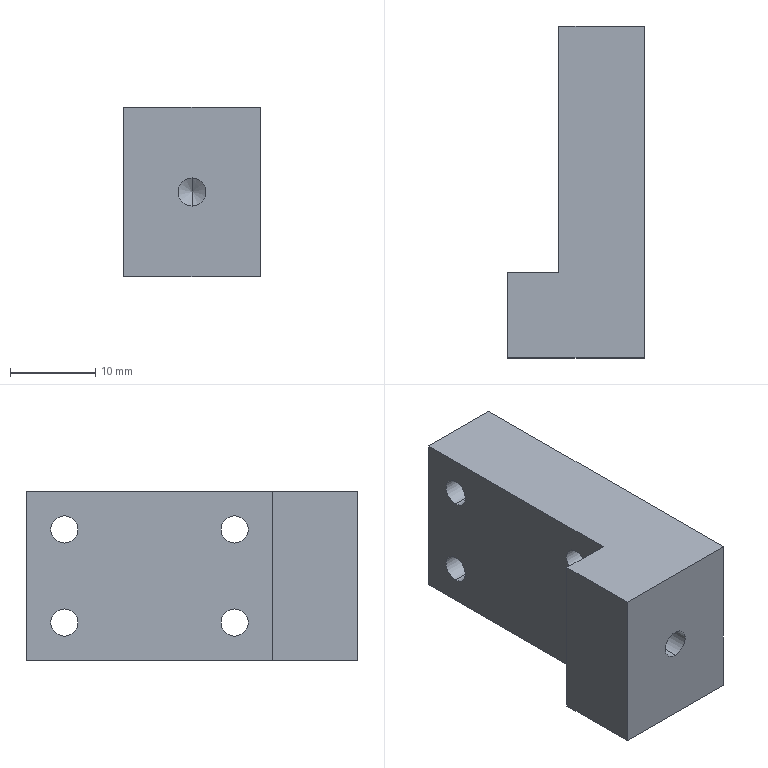Part | NX | features BREP 1 | 1 solid | 32 faces | box 16 x 39 x 19.94 mm | volume 8238 mm3 | cylinder 18 | plane 12 | cone 2 | commonest cylinder face diameters 3.2 x8 6.5 x8 3.3 x2
STEP:
#1=CARTESIAN_POINT('',(-8.,9.,11.62));
#2=VERTEX_POINT('',#1);
#3=CARTESIAN_POINT('',(-8.,9.,8.32));
#4=VERTEX_POINT('',#3);
#5=CARTESIAN_POINT('',(-8.,9.,9.97));
#6=DIRECTION('',(0.,-1.,0.));
#7=DIRECTION('',(0.,0.,-1.));
#8=AXIS2_PLACEMENT_3D('',#5,#6,#7);
#9=CIRCLE('',#8,1.65);
#10=EDGE_CURVE('',#2,#4,#9,.T.);
#11=ORIENTED_EDGE('',*,*,#10,.F.);
#12=CARTESIAN_POINT('',(-8.,1.,11.62));
#13=VERTEX_POINT('',#12);
#14=CARTESIAN_POINT('',(-8.,1.,11.62));
#15=DIRECTION('',(0.,-1.,0.));
#16=VECTOR('',#15,1000.);
#17=LINE('',#14,#16);
#18=EDGE_CURVE('',#2,#13,#17,.T.);
#19=ORIENTED_EDGE('',*,*,#18,.T.);
#20=CARTESIAN_POINT('',(-8.,1.,8.32));
#21=VERTEX_POINT('',#20);
#22=CARTESIAN_POINT('',(-8.,1.,9.97));
#23=DIRECTION('',(0.,-1.,0.));
#24=DIRECTION('',(0.,0.,-1.));
#25=AXIS2_PLACEMENT_3D('',#22,#23,#24);
#26=CIRCLE('',#25,1.65);
#27=EDGE_CURVE('',#13,#21,#26,.T.);
#28=ORIENTED_EDGE('',*,*,#27,.T.);
#29=CARTESIAN_POINT('',(-8.,1.,8.32));
#30=DIRECTION('',(0.,-1.,0.));
#31=VECTOR('',#30,1000.);
#32=LINE('',#29,#31);
#33=EDGE_CURVE('',#4,#21,#32,.T.);
#34=ORIENTED_EDGE('',*,*,#33,.F.);
#35=EDGE_LOOP('',(#11,#19,#28,#34));
#36=FACE_BOUND('',#35,.T.);
#37=CARTESIAN_POINT('',(-8.,1.,9.97));
#38=DIRECTION('',(0.,-1.,0.));
#39=DIRECTION('',(0.,0.,-1.));
#40=AXIS2_PLACEMENT_3D('',#37,#38,#39);
#41=CYLINDRICAL_SURFACE('',#40,1.65);
#42=ADVANCED_FACE('',(#36),#41,.F.);
#43=CARTESIAN_POINT('',(-8.,9.991,9.97));
#44=VERTEX_POINT('',#43);
#45=CARTESIAN_POINT('',(-8.,9.,8.32));
#46=DIRECTION('',(0.,-0.515,-0.8572));
#47=VECTOR('',#46,1000.);
#48=LINE('',#45,#47);
#49=EDGE_CURVE('',#44,#4,#48,.T.);
#50=ORIENTED_EDGE('',*,*,#49,.F.);
#51=CARTESIAN_POINT('',(-8.,9.,11.62));
#52=DIRECTION('',(0.,-0.515,0.8572));
#53=VECTOR('',#52,1000.);
#54=LINE('',#51,#53);
#55=EDGE_CURVE('',#44,#2,#54,.T.);
#56=ORIENTED_EDGE('',*,*,#55,.T.);
#57=ORIENTED_EDGE('',*,*,#10,.T.);
#58=EDGE_LOOP('',(#50,#56,#57));
#59=FACE_BOUND('',#58,.T.);
#60=CARTESIAN_POINT('',(-8.,9.,9.97));
#61=DIRECTION('',(0.,-1.,0.));
#62=DIRECTION('',(0.,0.,-1.));
#63=AXIS2_PLACEMENT_3D('',#60,#61,#62);
#64=CONICAL_SURFACE('',#63,1.65,1.03);
#65=ADVANCED_FACE('',(#59),#64,.F.);
#66=CARTESIAN_POINT('',(-3.4,35.5,18.69));
#67=VERTEX_POINT('',#66);
#68=CARTESIAN_POINT('',(-3.4,35.5,12.19));
#69=VERTEX_POINT('',#68);
#70=CARTESIAN_POINT('',(-3.4,35.5,15.44));
#71=DIRECTION('',(1.,0.,0.));
#72=DIRECTION('',(0.,0.,-1.));
#73=AXIS2_PLACEMENT_3D('',#70,#71,#72);
#74=CIRCLE('',#73,3.25);
#75=EDGE_CURVE('',#67,#69,#74,.T.);
#76=ORIENTED_EDGE('',*,*,#75,.F.);
#77=CARTESIAN_POINT('',(0.,35.5,18.69));
#78=VERTEX_POINT('',#77);
#79=CARTESIAN_POINT('',(0.,35.5,18.69));
#80=DIRECTION('',(1.,0.,0.));
#81=VECTOR('',#80,1000.);
#82=LINE('',#79,#81);
#83=EDGE_CURVE('',#67,#78,#82,.T.);
#84=ORIENTED_EDGE('',*,*,#83,.T.);
#85=CARTESIAN_POINT('',(0.,35.5,12.19));
#86=VERTEX_POINT('',#85);
#87=CARTESIAN_POINT('',(0.,35.5,15.44));
#88=DIRECTION('',(1.,0.,0.));
#89=DIRECTION('',(0.,0.,-1.));
#90=AXIS2_PLACEMENT_3D('',#87,#88,#89);
#91=CIRCLE('',#90,3.25);
#92=EDGE_CURVE('',#78,#86,#91,.T.);
#93=ORIENTED_EDGE('',*,*,#92,.T.);
#94=CARTESIAN_POINT('',(0.,35.5,12.19));
#95=DIRECTION('',(1.,0.,0.));
#96=VECTOR('',#95,1000.);
#97=LINE('',#94,#96);
#98=EDGE_CURVE('',#69,#86,#97,.T.);
#99=ORIENTED_EDGE('',*,*,#98,.F.);
#100=EDGE_LOOP('',(#76,#84,#93,#99));
#101=FACE_BOUND('',#100,.T.);
#102=CARTESIAN_POINT('',(0.,35.5,15.44));
#103=DIRECTION('',(1.,0.,0.));
#104=DIRECTION('',(0.,0.,-1.));
#105=AXIS2_PLACEMENT_3D('',#102,#103,#104);
#106=CYLINDRICAL_SURFACE('',#105,3.25);
#107=ADVANCED_FACE('',(#101),#106,.F.);
#108=CARTESIAN_POINT('',(-10.,35.5,17.04));
#109=VERTEX_POINT('',#108);
#110=CARTESIAN_POINT('',(-10.,35.5,13.84));
#111=VERTEX_POINT('',#110);
#112=CARTESIAN_POINT('',(-10.,35.5,15.44));
#113=DIRECTION('',(1.,0.,0.));
#114=DIRECTION('',(0.,0.,-1.));
#115=AXIS2_PLACEMENT_3D('',#112,#113,#114);
#116=CIRCLE('',#115,1.6);
#117=EDGE_CURVE('',#109,#111,#116,.T.);
#118=ORIENTED_EDGE('',*,*,#117,.F.);
#119=CARTESIAN_POINT('',(-3.4,35.5,17.04));
#120=VERTEX_POINT('',#119);
#121=CARTESIAN_POINT('',(0.,35.5,17.04));
#122=DIRECTION('',(1.,0.,0.));
#123=VECTOR('',#122,1000.);
#124=LINE('',#121,#123);
#125=EDGE_CURVE('',#109,#120,#124,.T.);
#126=ORIENTED_EDGE('',*,*,#125,.T.);
#127=CARTESIAN_POINT('',(-3.4,35.5,13.84));
#128=VERTEX_POINT('',#127);
#129=CARTESIAN_POINT('',(-3.4,35.5,15.44));
#130=DIRECTION('',(1.,0.,0.));
#131=DIRECTION('',(0.,0.,-1.));
#132=AXIS2_PLACEMENT_3D('',#129,#130,#131);
#133=CIRCLE('',#132,1.6);
#134=EDGE_CURVE('',#120,#128,#133,.T.);
#135=ORIENTED_EDGE('',*,*,#134,.T.);
#136=CARTESIAN_POINT('',(0.,35.5,13.84));
#137=DIRECTION('',(1.,0.,0.));
#138=VECTOR('',#137,1000.);
#139=LINE('',#136,#138);
#140=EDGE_CURVE('',#111,#128,#139,.T.);
#141=ORIENTED_EDGE('',*,*,#140,.F.);
#142=EDGE_LOOP('',(#118,#126,#135,#141));
#143=FACE_BOUND('',#142,.T.);
#144=CARTESIAN_POINT('',(0.,35.5,15.44));
#145=DIRECTION('',(1.,0.,0.));
#146=DIRECTION('',(0.,0.,-1.));
#147=AXIS2_PLACEMENT_3D('',#144,#145,#146);
#148=CYLINDRICAL_SURFACE('',#147,1.6);
#149=ADVANCED_FACE('',(#143),#148,.F.);
#150=CARTESIAN_POINT('',(-3.4,15.5,18.69));
#151=VERTEX_POINT('',#150);
#152=CARTESIAN_POINT('',(-3.4,15.5,12.19));
#153=VERTEX_POINT('',#152);
#154=CARTESIAN_POINT('',(-3.4,15.5,15.44));
#155=DIRECTION('',(1.,0.,0.));
#156=DIRECTION('',(0.,0.,-1.));
#157=AXIS2_PLACEMENT_3D('',#154,#155,#156);
#158=CIRCLE('',#157,3.25);
#159=EDGE_CURVE('',#151,#153,#158,.T.);
#160=ORIENTED_EDGE('',*,*,#159,.F.);
#161=CARTESIAN_POINT('',(0.,15.5,18.69));
#162=VERTEX_POINT('',#161);
#163=CARTESIAN_POINT('',(0.,15.5,18.69));
#164=DIRECTION('',(1.,0.,0.));
#165=VECTOR('',#164,1000.);
#166=LINE('',#163,#165);
#167=EDGE_CURVE('',#151,#162,#166,.T.);
#168=ORIENTED_EDGE('',*,*,#167,.T.);
#169=CARTESIAN_POINT('',(0.,15.5,12.19));
#170=VERTEX_POINT('',#169);
#171=CARTESIAN_POINT('',(0.,15.5,15.44));
#172=DIRECTION('',(1.,0.,0.));
#173=DIRECTION('',(0.,0.,-1.));
#174=AXIS2_PLACEMENT_3D('',#171,#172,#173);
#175=CIRCLE('',#174,3.25);
#176=EDGE_CURVE('',#162,#170,#175,.T.);
#177=ORIENTED_EDGE('',*,*,#176,.T.);
#178=CARTESIAN_POINT('',(0.,15.5,12.19));
#179=DIRECTION('',(1.,0.,0.));
#180=VECTOR('',#179,1000.);
#181=LINE('',#178,#180);
#182=EDGE_CURVE('',#153,#170,#181,.T.);
#183=ORIENTED_EDGE('',*,*,#182,.F.);
#184=EDGE_LOOP('',(#160,#168,#177,#183));
#185=FACE_BOUND('',#184,.T.);
#186=CARTESIAN_POINT('',(0.,15.5,15.44));
#187=DIRECTION('',(1.,0.,0.));
#188=DIRECTION('',(0.,0.,-1.));
#189=AXIS2_PLACEMENT_3D('',#186,#187,#188);
#190=CYLINDRICAL_SURFACE('',#189,3.25);
#191=ADVANCED_FACE('',(#185),#190,.F.);
#192=CARTESIAN_POINT('',(-10.,15.5,17.04));
#193=VERTEX_POINT('',#192);
#194=CARTESIAN_POINT('',(-10.,15.5,13.84));
#195=VERTEX_POINT('',#194);
#196=CARTESIAN_POINT('',(-10.,15.5,15.44));
#197=DIRECTION('',(1.,0.,0.));
#198=DIRECTION('',(0.,0.,-1.));
#199=AXIS2_PLACEMENT_3D('',#196,#197,#198);
#200=CIRCLE('',#199,1.6);
#201=EDGE_CURVE('',#193,#195,#200,.T.);
#202=ORIENTED_EDGE('',*,*,#201,.F.);
#203=CARTESIAN_POINT('',(-3.4,15.5,17.04));
#204=VERTEX_POINT('',#203);
#205=CARTESIAN_POINT('',(0.,15.5,17.04));
#206=DIRECTION('',(1.,0.,0.));
#207=VECTOR('',#206,1000.);
#208=LINE('',#205,#207);
#209=EDGE_CURVE('',#193,#204,#208,.T.);
#210=ORIENTED_EDGE('',*,*,#209,.T.);
#211=CARTESIAN_POINT('',(-3.4,15.5,13.84));
#212=VERTEX_POINT('',#211);
#213=CARTESIAN_POINT('',(-3.4,15.5,15.44));
#214=DIRECTION('',(1.,0.,0.));
#215=DIRECTION('',(0.,0.,-1.));
#216=AXIS2_PLACEMENT_3D('',#213,#214,#215);
#217=CIRCLE('',#216,1.6);
#218=EDGE_CURVE('',#204,#212,#217,.T.);
#219=ORIENTED_EDGE('',*,*,#218,.T.);
#220=CARTESIAN_POINT('',(0.,15.5,13.84));
#221=DIRECTION('',(1.,0.,0.));
#222=VECTOR('',#221,1000.);
#223=LINE('',#220,#222);
#224=EDGE_CURVE('',#195,#212,#223,.T.);
#225=ORIENTED_EDGE('',*,*,#224,.F.);
#226=EDGE_LOOP('',(#202,#210,#219,#225));
#227=FACE_BOUND('',#226,.T.);
#228=CARTESIAN_POINT('',(0.,15.5,15.44));
#229=DIRECTION('',(1.,0.,0.));
#230=DIRECTION('',(0.,0.,-1.));
#231=AXIS2_PLACEMENT_3D('',#228,#229,#230);
#232=CYLINDRICAL_SURFACE('',#231,1.6);
#233=ADVANCED_FACE('',(#227),#232,.F.);
#234=CARTESIAN_POINT('',(-3.4,35.5,7.75));
#235=VERTEX_POINT('',#234);
#236=CARTESIAN_POINT('',(-3.4,35.5,1.25));
#237=VERTEX_POINT('',#236);
#238=CARTESIAN_POINT('',(-3.4,35.5,4.5));
#239=DIRECTION('',(1.,0.,0.));
#240=DIRECTION('',(0.,0.,-1.));
#241=AXIS2_PLACEMENT_3D('',#238,#239,#240);
#242=CIRCLE('',#241,3.25);
#243=EDGE_CURVE('',#235,#237,#242,.T.);
#244=ORIENTED_EDGE('',*,*,#243,.F.);
#245=CARTESIAN_POINT('',(0.,35.5,7.75));
#246=VERTEX_POINT('',#245);
#247=CARTESIAN_POINT('',(0.,35.5,7.75));
#248=DIRECTION('',(1.,0.,0.));
#249=VECTOR('',#248,1000.);
#250=LINE('',#247,#249);
#251=EDGE_CURVE('',#235,#246,#250,.T.);
#252=ORIENTED_EDGE('',*,*,#251,.T.);
#253=CARTESIAN_POINT('',(0.,35.5,1.25));
#254=VERTEX_POINT('',#253);
#255=CARTESIAN_POINT('',(0.,35.5,4.5));
#256=DIRECTION('',(1.,0.,0.));
#257=DIRECTION('',(0.,0.,-1.));
#258=AXIS2_PLACEMENT_3D('',#255,#256,#257);
#259=CIRCLE('',#258,3.25);
#260=EDGE_CURVE('',#246,#254,#259,.T.);
#261=ORIENTED_EDGE('',*,*,#260,.T.);
#262=CARTESIAN_POINT('',(0.,35.5,1.25));
#263=DIRECTION('',(1.,0.,0.));
#264=VECTOR('',#263,1000.);
#265=LINE('',#262,#264);
#266=EDGE_CURVE('',#237,#254,#265,.T.);
#267=ORIENTED_EDGE('',*,*,#266,.F.);
#268=EDGE_LOOP('',(#244,#252,#261,#267));
#269=FACE_BOUND('',#268,.T.);
#270=CARTESIAN_POINT('',(0.,35.5,4.5));
#271=DIRECTION('',(1.,0.,0.));
#272=DIRECTION('',(0.,0.,-1.));
#273=AXIS2_PLACEMENT_3D('',#270,#271,#272);
#274=CYLINDRICAL_SURFACE('',#273,3.25);
#275=ADVANCED_FACE('',(#269),#274,.F.);
#276=CARTESIAN_POINT('',(-10.,35.5,6.1));
#277=VERTEX_POINT('',#276);
#278=CARTESIAN_POINT('',(-10.,35.5,2.9));
#279=VERTEX_POINT('',#278);
#280=CARTESIAN_POINT('',(-10.,35.5,4.5));
#281=DIRECTION('',(1.,0.,0.));
#282=DIRECTION('',(0.,0.,-1.));
#283=AXIS2_PLACEMENT_3D('',#280,#281,#282);
#284=CIRCLE('',#283,1.6);
#285=EDGE_CURVE('',#277,#279,#284,.T.);
#286=ORIENTED_EDGE('',*,*,#285,.F.);
#287=CARTESIAN_POINT('',(-3.4,35.5,6.1));
#288=VERTEX_POINT('',#287);
#289=CARTESIAN_POINT('',(0.,35.5,6.1));
#290=DIRECTION('',(1.,0.,0.));
#291=VECTOR('',#290,1000.);
#292=LINE('',#289,#291);
#293=EDGE_CURVE('',#277,#288,#292,.T.);
#294=ORIENTED_EDGE('',*,*,#293,.T.);
#295=CARTESIAN_POINT('',(-3.4,35.5,2.9));
#296=VERTEX_POINT('',#295);
#297=CARTESIAN_POINT('',(-3.4,35.5,4.5));
#298=DIRECTION('',(1.,0.,0.));
#299=DIRECTION('',(0.,0.,-1.));
#300=AXIS2_PLACEMENT_3D('',#297,#298,#299);
#301=CIRCLE('',#300,1.6);
#302=EDGE_CURVE('',#288,#296,#301,.T.);
#303=ORIENTED_EDGE('',*,*,#302,.T.);
#304=CARTESIAN_POINT('',(0.,35.5,2.9));
#305=DIRECTION('',(1.,0.,0.));
#306=VECTOR('',#305,1000.);
#307=LINE('',#304,#306);
#308=EDGE_CURVE('',#279,#296,#307,.T.);
#309=ORIENTED_EDGE('',*,*,#308,.F.);
#310=EDGE_LOOP('',(#286,#294,#303,#309));
#311=FACE_BOUND('',#310,.T.);
#312=CARTESIAN_POINT('',(0.,35.5,4.5));
#313=DIRECTION('',(1.,0.,0.));
#314=DIRECTION('',(0.,0.,-1.));
#315=AXIS2_PLACEMENT_3D('',#312,#313,#314);
#316=CYLINDRICAL_SURFACE('',#315,1.6);
#317=ADVANCED_FACE('',(#311),#316,.F.);
#318=CARTESIAN_POINT('',(-3.4,15.5,7.75));
#319=VERTEX_POINT('',#318);
#320=CARTESIAN_POINT('',(-3.4,15.5,1.25));
#321=VERTEX_POINT('',#320);
#322=CARTESIAN_POINT('',(-3.4,15.5,4.5));
#323=DIRECTION('',(1.,0.,0.));
#324=DIRECTION('',(0.,0.,-1.));
#325=AXIS2_PLACEMENT_3D('',#322,#323,#324);
#326=CIRCLE('',#325,3.25);
#327=EDGE_CURVE('',#319,#321,#326,.T.);
#328=ORIENTED_EDGE('',*,*,#327,.F.);
#329=CARTESIAN_POINT('',(0.,15.5,7.75));
#330=VERTEX_POINT('',#329);
#331=CARTESIAN_POINT('',(0.,15.5,7.75));
#332=DIRECTION('',(1.,0.,0.));
#333=VECTOR('',#332,1000.);
#334=LINE('',#331,#333);
#335=EDGE_CURVE('',#319,#330,#334,.T.);
#336=ORIENTED_EDGE('',*,*,#335,.T.);
#337=CARTESIAN_POINT('',(0.,15.5,1.25));
#338=VERTEX_POINT('',#337);
#339=CARTESIAN_POINT('',(0.,15.5,4.5));
#340=DIRECTION('',(1.,0.,0.));
#341=DIRECTION('',(0.,0.,-1.));
#342=AXIS2_PLACEMENT_3D('',#339,#340,#341);
#343=CIRCLE('',#342,3.25);
#344=EDGE_CURVE('',#330,#338,#343,.T.);
#345=ORIENTED_EDGE('',*,*,#344,.T.);
#346=CARTESIAN_POINT('',(0.,15.5,1.25));
#347=DIRECTION('',(1.,0.,0.));
#348=VECTOR('',#347,1000.);
#349=LINE('',#346,#348);
#350=EDGE_CURVE('',#321,#338,#349,.T.);
#351=ORIENTED_EDGE('',*,*,#350,.F.);
#352=EDGE_LOOP('',(#328,#336,#345,#351));
#353=FACE_BOUND('',#352,.T.);
#354=CARTESIAN_POINT('',(0.,15.5,4.5));
#355=DIRECTION('',(1.,0.,0.));
#356=DIRECTION('',(0.,0.,-1.));
#357=AXIS2_PLACEMENT_3D('',#354,#355,#356);
#358=CYLINDRICAL_SURFACE('',#357,3.25);
#359=ADVANCED_FACE('',(#353),#358,.F.);
#360=CARTESIAN_POINT('',(-10.,15.5,6.1));
#361=VERTEX_POINT('',#360);
#362=CARTESIAN_POINT('',(-10.,15.5,2.9));
#363=VERTEX_POINT('',#362);
#364=CARTESIAN_POINT('',(-10.,15.5,4.5));
#365=DIRECTION('',(1.,0.,0.));
#366=DIRECTION('',(0.,0.,-1.));
#367=AXIS2_PLACEMENT_3D('',#364,#365,#366);
#368=CIRCLE('',#367,1.6);
#369=EDGE_CURVE('',#361,#363,#368,.T.);
#370=ORIENTED_EDGE('',*,*,#369,.F.);
#371=CARTESIAN_POINT('',(-3.4,15.5,6.1));
#372=VERTEX_POINT('',#371);
#373=CARTESIAN_POINT('',(0.,15.5,6.1));
#374=DIRECTION('',(1.,0.,0.));
#375=VECTOR('',#374,1000.);
#376=LINE('',#373,#375);
#377=EDGE_CURVE('',#361,#372,#376,.T.);
#378=ORIENTED_EDGE('',*,*,#377,.T.);
#379=CARTESIAN_POINT('',(-3.4,15.5,2.9));
#380=VERTEX_POINT('',#379);
#381=CARTESIAN_POINT('',(-3.4,15.5,4.5));
#382=DIRECTION('',(1.,0.,0.));
#383=DIRECTION('',(0.,0.,-1.));
#384=AXIS2_PLACEMENT_3D('',#381,#382,#383);
#385=CIRCLE('',#384,1.6);
#386=EDGE_CURVE('',#372,#380,#385,.T.);
#387=ORIENTED_EDGE('',*,*,#386,.T.);
#388=CARTESIAN_POINT('',(0.,15.5,2.9));
#389=DIRECTION('',(1.,0.,0.));
#390=VECTOR('',#389,1000.);
#391=LINE('',#388,#390);
#392=EDGE_CURVE('',#363,#380,#391,.T.);
#393=ORIENTED_EDGE('',*,*,#392,.F.);
#394=EDGE_LOOP('',(#370,#378,#387,#393));
#395=FACE_BOUND('',#394,.T.);
#396=CARTESIAN_POINT('',(0.,15.5,4.5));
#397=DIRECTION('',(1.,0.,0.));
#398=DIRECTION('',(0.,0.,-1.));
#399=AXIS2_PLACEMENT_3D('',#396,#397,#398);
#400=CYLINDRICAL_SURFACE('',#399,1.6);
#401=ADVANCED_FACE('',(#395),#400,.F.);
#402=CARTESIAN_POINT('',(0.,1.,0.));
#403=VERTEX_POINT('',#402);
#404=CARTESIAN_POINT('',(0.,1.,19.94));
#405=VERTEX_POINT('',#404);
#406=CARTESIAN_POINT('',(0.,1.,19.94));
#407=DIRECTION('',(0.,0.,1.));
#408=VECTOR('',#407,1000.);
#409=LINE('',#406,#408);
#410=EDGE_CURVE('',#403,#405,#409,.T.);
#411=ORIENTED_EDGE('',*,*,#410,.F.);
#412=CARTESIAN_POINT('',(0.,40.,0.));
#413=VERTEX_POINT('',#412);
#414=CARTESIAN_POINT('',(0.,0.,0.));
#415=DIRECTION('',(0.,-1.,0.));
#416=VECTOR('',#415,1000.);
#417=LINE('',#414,#416);
#418=EDGE_CURVE('',#413,#403,#417,.T.);
#419=ORIENTED_EDGE('',*,*,#418,.F.);
#420=CARTESIAN_POINT('',(0.,40.,19.94));
#421=VERTEX_POINT('',#420);
#422=CARTESIAN_POINT('',(0.,40.,19.94));
#423=DIRECTION('',(0.,0.,-1.));
#424=VECTOR('',#423,1000.);
#425=LINE('',#422,#424);
#426=EDGE_CURVE('',#421,#413,#425,.T.);
#427=ORIENTED_EDGE('',*,*,#426,.F.);
#428=CARTESIAN_POINT('',(0.,0.,19.94));
#429=DIRECTION('',(0.,-1.,0.));
#430=VECTOR('',#429,1000.);
#431=LINE('',#428,#430);
#432=EDGE_CURVE('',#421,#405,#431,.T.);
#433=ORIENTED_EDGE('',*,*,#432,.T.);
#434=EDGE_LOOP('',(#411,#419,#427,#433));
#435=FACE_BOUND('',#434,.T.);
#436=CARTESIAN_POINT('',(0.,35.5,15.44));
#437=DIRECTION('',(1.,0.,0.));
#438=DIRECTION('',(0.,0.,-1.));
#439=AXIS2_PLACEMENT_3D('',#436,#437,#438);
#440=CIRCLE('',#439,3.25);
#441=EDGE_CURVE('',#86,#78,#440,.T.);
#442=ORIENTED_EDGE('',*,*,#441,.F.);
#443=ORIENTED_EDGE('',*,*,#92,.F.);
#444=EDGE_LOOP('',(#442,#443));
#445=FACE_BOUND('',#444,.T.);
#446=CARTESIAN_POINT('',(0.,15.5,15.44));
#447=DIRECTION('',(1.,0.,0.));
#448=DIRECTION('',(0.,0.,-1.));
#449=AXIS2_PLACEMENT_3D('',#446,#447,#448);
#450=CIRCLE('',#449,3.25);
#451=EDGE_CURVE('',#170,#162,#450,.T.);
#452=ORIENTED_EDGE('',*,*,#451,.F.);
#453=ORIENTED_EDGE('',*,*,#176,.F.);
#454=EDGE_LOOP('',(#452,#453));
#455=FACE_BOUND('',#454,.T.);
#456=CARTESIAN_POINT('',(0.,35.5,4.5));
#457=DIRECTION('',(1.,0.,0.));
#458=DIRECTION('',(0.,0.,-1.));
#459=AXIS2_PLACEMENT_3D('',#456,#457,#458);
#460=CIRCLE('',#459,3.25);
#461=EDGE_CURVE('',#254,#246,#460,.T.);
#462=ORIENTED_EDGE('',*,*,#461,.F.);
#463=ORIENTED_EDGE('',*,*,#260,.F.);
#464=EDGE_LOOP('',(#462,#463));
#465=FACE_BOUND('',#464,.T.);
#466=CARTESIAN_POINT('',(0.,15.5,4.5));
#467=DIRECTION('',(1.,0.,0.));
#468=DIRECTION('',(0.,0.,-1.));
#469=AXIS2_PLACEMENT_3D('',#466,#467,#468);
#470=CIRCLE('',#469,3.25);
#471=EDGE_CURVE('',#338,#330,#470,.T.);
#472=ORIENTED_EDGE('',*,*,#471,.F.);
#473=ORIENTED_EDGE('',*,*,#344,.F.);
#474=EDGE_LOOP('',(#472,#473));
#475=FACE_BOUND('',#474,.T.);
#476=CARTESIAN_POINT('',(0.,0.,19.94));
#477=DIRECTION('',(1.,0.,0.));
#478=DIRECTION('',(0.,1.,0.));
#479=AXIS2_PLACEMENT_3D('',#476,#477,#478);
#480=PLANE('',#479);
#481=ADVANCED_FACE('',(#435,#445,#455,#465,#475),#480,.T.);
#482=CARTESIAN_POINT('',(-10.,40.,19.94));
#483=VERTEX_POINT('',#482);
#484=CARTESIAN_POINT('',(-10.,40.,0.));
#485=VERTEX_POINT('',#484);
#486=CARTESIAN_POINT('',(-10.,40.,19.94));
#487=DIRECTION('',(0.,0.,-1.));
#488=VECTOR('',#487,1000.);
#489=LINE('',#486,#488);
#490=EDGE_CURVE('',#483,#485,#489,.T.);
#491=ORIENTED_EDGE('',*,*,#490,.F.);
#492=CARTESIAN_POINT('',(-10.,40.,19.94));
#493=DIRECTION('',(1.,0.,0.));
#494=VECTOR('',#493,1000.);
#495=LINE('',#492,#494);
#496=EDGE_CURVE('',#483,#421,#495,.T.);
#497=ORIENTED_EDGE('',*,*,#496,.T.);
#498=ORIENTED_EDGE('',*,*,#426,.T.);
#499=CARTESIAN_POINT('',(-10.,40.,0.));
#500=DIRECTION('',(1.,0.,0.));
#501=VECTOR('',#500,1000.);
#502=LINE('',#499,#501);
#503=EDGE_CURVE('',#485,#413,#502,.T.);
#504=ORIENTED_EDGE('',*,*,#503,.F.);
#505=EDGE_LOOP('',(#491,#497,#498,#504));
#506=FACE_BOUND('',#505,.T.);
#507=CARTESIAN_POINT('',(-10.,40.,19.94));
#508=DIRECTION('',(0.,1.,0.));
#509=DIRECTION('',(1.,0.,0.));
#510=AXIS2_PLACEMENT_3D('',#507,#508,#509);
#511=PLANE('',#510);
#512=ADVANCED_FACE('',(#506),#511,.T.);
#513=CARTESIAN_POINT('',(-16.,11.,0.));
#514=VERTEX_POINT('',#513);
#515=CARTESIAN_POINT('',(-16.,1.,0.));
#516=VERTEX_POINT('',#515);
#517=CARTESIAN_POINT('',(-16.,0.,0.));
#518=DIRECTION('',(0.,-1.,0.));
#519=VECTOR('',#518,1000.);
#520=LINE('',#517,#519);
#521=EDGE_CURVE('',#514,#516,#520,.T.);
#522=ORIENTED_EDGE('',*,*,#521,.T.);
#523=CARTESIAN_POINT('',(-16.,1.,19.94));
#524=VERTEX_POINT('',#523);
#525=CARTESIAN_POINT('',(-16.,1.,19.94));
#526=DIRECTION('',(0.,0.,1.));
#527=VECTOR('',#526,1000.);
#528=LINE('',#525,#527);
#529=EDGE_CURVE('',#516,#524,#528,.T.);
#530=ORIENTED_EDGE('',*,*,#529,.T.);
#531=CARTESIAN_POINT('',(-16.,11.,19.94));
#532=VERTEX_POINT('',#531);
#533=CARTESIAN_POINT('',(-16.,0.,19.94));
#534=DIRECTION('',(0.,-1.,0.));
#535=VECTOR('',#534,1000.);
#536=LINE('',#533,#535);
#537=EDGE_CURVE('',#532,#524,#536,.T.);
#538=ORIENTED_EDGE('',*,*,#537,.F.);
#539=CARTESIAN_POINT('',(-16.,11.,19.94));
#540=DIRECTION('',(0.,0.,-1.));
#541=VECTOR('',#540,1000.);
#542=LINE('',#539,#541);
#543=EDGE_CURVE('',#532,#514,#542,.T.);
#544=ORIENTED_EDGE('',*,*,#543,.T.);
#545=EDGE_LOOP('',(#522,#530,#538,#544));
#546=FACE_BOUND('',#545,.T.);
#547=CARTESIAN_POINT('',(-16.,0.,19.94));
#548=DIRECTION('',(1.,0.,0.));
#549=DIRECTION('',(0.,1.,0.));
#550=AXIS2_PLACEMENT_3D('',#547,#548,#549);
#551=PLANE('',#550);
#552=ADVANCED_FACE('',(#546),#551,.F.);
#553=ORIENTED_EDGE('',*,*,#537,.T.);
#554=CARTESIAN_POINT('',(-49.363,1.,19.94));
#555=DIRECTION('',(-1.,0.,0.));
#556=VECTOR('',#555,1000.);
#557=LINE('',#554,#556);
#558=EDGE_CURVE('',#405,#524,#557,.T.);
#559=ORIENTED_EDGE('',*,*,#558,.F.);
#560=ORIENTED_EDGE('',*,*,#432,.F.);
#561=ORIENTED_EDGE('',*,*,#496,.F.);
#562=CARTESIAN_POINT('',(-10.,11.,19.94));
#563=VERTEX_POINT('',#562);
#564=CARTESIAN_POINT('',(-10.,11.,19.94));
#565=DIRECTION('',(0.,1.,0.));
#566=VECTOR('',#565,1000.);
#567=LINE('',#564,#566);
#568=EDGE_CURVE('',#563,#483,#567,.T.);
#569=ORIENTED_EDGE('',*,*,#568,.F.);
#570=CARTESIAN_POINT('',(-6.,11.,19.94));
#571=DIRECTION('',(1.,0.,0.));
#572=VECTOR('',#571,1000.);
#573=LINE('',#570,#572);
#574=EDGE_CURVE('',#532,#563,#573,.T.);
#575=ORIENTED_EDGE('',*,*,#574,.F.);
#576=EDGE_LOOP('',(#553,#559,#560,#561,#569,#575));
#577=FACE_BOUND('',#576,.T.);
#578=CARTESIAN_POINT('',(0.,0.,19.94));
#579=DIRECTION('',(0.,0.,-1.));
#580=DIRECTION('',(0.,-1.,0.));
#581=AXIS2_PLACEMENT_3D('',#578,#579,#580);
#582=PLANE('',#581);
#583=ADVANCED_FACE('',(#577),#582,.F.);
#584=CARTESIAN_POINT('',(0.,1.,0.));
#585=DIRECTION('',(1.,0.,0.));
#586=VECTOR('',#585,1000.);
#587=LINE('',#584,#586);
#588=EDGE_CURVE('',#516,#403,#587,.T.);
#589=ORIENTED_EDGE('',*,*,#588,.F.);
#590=ORIENTED_EDGE('',*,*,#521,.F.);
#591=CARTESIAN_POINT('',(-10.,11.,0.));
#592=VERTEX_POINT('',#591);
#593=CARTESIAN_POINT('',(0.,11.,0.));
#594=DIRECTION('',(-1.,0.,0.));
#595=VECTOR('',#594,1000.);
#596=LINE('',#593,#595);
#597=EDGE_CURVE('',#592,#514,#596,.T.);
#598=ORIENTED_EDGE('',*,*,#597,.F.);
#599=CARTESIAN_POINT('',(-10.,11.,0.));
#600=DIRECTION('',(0.,1.,0.));
#601=VECTOR('',#600,1000.);
#602=LINE('',#599,#601);
#603=EDGE_CURVE('',#592,#485,#602,.T.);
#604=ORIENTED_EDGE('',*,*,#603,.T.);
#605=ORIENTED_EDGE('',*,*,#503,.T.);
#606=ORIENTED_EDGE('',*,*,#418,.T.);
#607=EDGE_LOOP('',(#589,#590,#598,#604,#605,#606));
#608=FACE_BOUND('',#607,.T.);
#609=CARTESIAN_POINT('',(0.,0.,0.));
#610=DIRECTION('',(0.,0.,-1.));
#611=DIRECTION('',(0.,-1.,0.));
#612=AXIS2_PLACEMENT_3D('',#609,#610,#611);
#613=PLANE('',#612);
#614=ADVANCED_FACE('',(#608),#613,.T.);
#615=ORIENTED_EDGE('',*,*,#574,.T.);
#616=CARTESIAN_POINT('',(-10.,11.,0.));
#617=DIRECTION('',(0.,0.,1.));
#618=VECTOR('',#617,1000.);
#619=LINE('',#616,#618);
#620=EDGE_CURVE('',#592,#563,#619,.T.);
#621=ORIENTED_EDGE('',*,*,#620,.F.);
#622=ORIENTED_EDGE('',*,*,#597,.T.);
#623=ORIENTED_EDGE('',*,*,#543,.F.);
#624=EDGE_LOOP('',(#615,#621,#622,#623));
#625=FACE_BOUND('',#624,.T.);
#626=CARTESIAN_POINT('',(-6.,11.,0.));
#627=DIRECTION('',(0.,-1.,0.));
#628=DIRECTION('',(0.,0.,-1.));
#629=AXIS2_PLACEMENT_3D('',#626,#627,#628);
#630=PLANE('',#629);
#631=ADVANCED_FACE('',(#625),#630,.F.);
#632=ORIENTED_EDGE('',*,*,#490,.T.);
#633=ORIENTED_EDGE('',*,*,#603,.F.);
#634=ORIENTED_EDGE('',*,*,#620,.T.);
#635=ORIENTED_EDGE('',*,*,#568,.T.);
#636=EDGE_LOOP('',(#632,#633,#634,#635));
#637=FACE_BOUND('',#636,.T.);
#638=CARTESIAN_POINT('',(-10.,35.5,15.44));
#639=DIRECTION('',(1.,0.,0.));
#640=DIRECTION('',(0.,0.,-1.));
#641=AXIS2_PLACEMENT_3D('',#638,#639,#640);
#642=CIRCLE('',#641,1.6);
#643=EDGE_CURVE('',#111,#109,#642,.T.);
#644=ORIENTED_EDGE('',*,*,#643,.T.);
#645=ORIENTED_EDGE('',*,*,#117,.T.);
#646=EDGE_LOOP('',(#644,#645));
#647=FACE_BOUND('',#646,.T.);
#648=CARTESIAN_POINT('',(-10.,15.5,15.44));
#649=DIRECTION('',(1.,0.,0.));
#650=DIRECTION('',(0.,0.,-1.));
#651=AXIS2_PLACEMENT_3D('',#648,#649,#650);
#652=CIRCLE('',#651,1.6);
#653=EDGE_CURVE('',#195,#193,#652,.T.);
#654=ORIENTED_EDGE('',*,*,#653,.T.);
#655=ORIENTED_EDGE('',*,*,#201,.T.);
#656=EDGE_LOOP('',(#654,#655));
#657=FACE_BOUND('',#656,.T.);
#658=CARTESIAN_POINT('',(-10.,35.5,4.5));
#659=DIRECTION('',(1.,0.,0.));
#660=DIRECTION('',(0.,0.,-1.));
#661=AXIS2_PLACEMENT_3D('',#658,#659,#660);
#662=CIRCLE('',#661,1.6);
#663=EDGE_CURVE('',#279,#277,#662,.T.);
#664=ORIENTED_EDGE('',*,*,#663,.T.);
#665=ORIENTED_EDGE('',*,*,#285,.T.);
#666=EDGE_LOOP('',(#664,#665));
#667=FACE_BOUND('',#666,.T.);
#668=CARTESIAN_POINT('',(-10.,15.5,4.5));
#669=DIRECTION('',(1.,0.,0.));
#670=DIRECTION('',(0.,0.,-1.));
#671=AXIS2_PLACEMENT_3D('',#668,#669,#670);
#672=CIRCLE('',#671,1.6);
#673=EDGE_CURVE('',#363,#361,#672,.T.);
#674=ORIENTED_EDGE('',*,*,#673,.T.);
#675=ORIENTED_EDGE('',*,*,#369,.T.);
#676=EDGE_LOOP('',(#674,#675));
#677=FACE_BOUND('',#676,.T.);
#678=CARTESIAN_POINT('',(-10.,11.,0.));
#679=DIRECTION('',(1.,0.,0.));
#680=DIRECTION('',(0.,1.,0.));
#681=AXIS2_PLACEMENT_3D('',#678,#679,#680);
#682=PLANE('',#681);
#683=ADVANCED_FACE('',(#637,#647,#657,#667,#677),#682,.F.);
#684=ORIENTED_EDGE('',*,*,#377,.F.);
#685=ORIENTED_EDGE('',*,*,#673,.F.);
#686=ORIENTED_EDGE('',*,*,#392,.T.);
#687=CARTESIAN_POINT('',(-3.4,15.5,4.5));
#688=DIRECTION('',(1.,0.,0.));
#689=DIRECTION('',(0.,0.,-1.));
#690=AXIS2_PLACEMENT_3D('',#687,#688,#689);
#691=CIRCLE('',#690,1.6);
#692=EDGE_CURVE('',#380,#372,#691,.T.);
#693=ORIENTED_EDGE('',*,*,#692,.T.);
#694=EDGE_LOOP('',(#684,#685,#686,#693));
#695=FACE_BOUND('',#694,.T.);
#696=CARTESIAN_POINT('',(0.,15.5,4.5));
#697=DIRECTION('',(1.,0.,0.));
#698=DIRECTION('',(0.,0.,-1.));
#699=AXIS2_PLACEMENT_3D('',#696,#697,#698);
#700=CYLINDRICAL_SURFACE('',#699,1.6);
#701=ADVANCED_FACE('',(#695),#700,.F.);
#702=CARTESIAN_POINT('',(-3.4,15.5,4.5));
#703=DIRECTION('',(1.,0.,0.));
#704=DIRECTION('',(0.,0.,-1.));
#705=AXIS2_PLACEMENT_3D('',#702,#703,#704);
#706=CIRCLE('',#705,3.25);
#707=EDGE_CURVE('',#321,#319,#706,.T.);
#708=ORIENTED_EDGE('',*,*,#707,.T.);
#709=ORIENTED_EDGE('',*,*,#327,.T.);
#710=EDGE_LOOP('',(#708,#709));
#711=FACE_BOUND('',#710,.T.);
#712=ORIENTED_EDGE('',*,*,#692,.F.);
#713=ORIENTED_EDGE('',*,*,#386,.F.);
#714=EDGE_LOOP('',(#712,#713));
#715=FACE_BOUND('',#714,.T.);
#716=CARTESIAN_POINT('',(-3.4,17.1,4.5));
#717=DIRECTION('',(-1.,0.,0.));
#718=DIRECTION('',(0.,0.,1.));
#719=AXIS2_PLACEMENT_3D('',#716,#717,#718);
#720=PLANE('',#719);
#721=ADVANCED_FACE('',(#711,#715),#720,.F.);
#722=ORIENTED_EDGE('',*,*,#335,.F.);
#723=ORIENTED_EDGE('',*,*,#707,.F.);
#724=ORIENTED_EDGE('',*,*,#350,.T.);
#725=ORIENTED_EDGE('',*,*,#471,.T.);
#726=EDGE_LOOP('',(#722,#723,#724,#725));
#727=FACE_BOUND('',#726,.T.);
#728=CARTESIAN_POINT('',(0.,15.5,4.5));
#729=DIRECTION('',(1.,0.,0.));
#730=DIRECTION('',(0.,0.,-1.));
#731=AXIS2_PLACEMENT_3D('',#728,#729,#730);
#732=CYLINDRICAL_SURFACE('',#731,3.25);
#733=ADVANCED_FACE('',(#727),#732,.F.);
#734=ORIENTED_EDGE('',*,*,#293,.F.);
#735=ORIENTED_EDGE('',*,*,#663,.F.);
#736=ORIENTED_EDGE('',*,*,#308,.T.);
#737=CARTESIAN_POINT('',(-3.4,35.5,4.5));
#738=DIRECTION('',(1.,0.,0.));
#739=DIRECTION('',(0.,0.,-1.));
#740=AXIS2_PLACEMENT_3D('',#737,#738,#739);
#741=CIRCLE('',#740,1.6);
#742=EDGE_CURVE('',#296,#288,#741,.T.);
#743=ORIENTED_EDGE('',*,*,#742,.T.);
#744=EDGE_LOOP('',(#734,#735,#736,#743));
#745=FACE_BOUND('',#744,.T.);
#746=CARTESIAN_POINT('',(0.,35.5,4.5));
#747=DIRECTION('',(1.,0.,0.));
#748=DIRECTION('',(0.,0.,-1.));
#749=AXIS2_PLACEMENT_3D('',#746,#747,#748);
#750=CYLINDRICAL_SURFACE('',#749,1.6);
#751=ADVANCED_FACE('',(#745),#750,.F.);
#752=CARTESIAN_POINT('',(-3.4,35.5,4.5));
#753=DIRECTION('',(1.,0.,0.));
#754=DIRECTION('',(0.,0.,-1.));
#755=AXIS2_PLACEMENT_3D('',#752,#753,#754);
#756=CIRCLE('',#755,3.25);
#757=EDGE_CURVE('',#237,#235,#756,.T.);
#758=ORIENTED_EDGE('',*,*,#757,.T.);
#759=ORIENTED_EDGE('',*,*,#243,.T.);
#760=EDGE_LOOP('',(#758,#759));
#761=FACE_BOUND('',#760,.T.);
#762=ORIENTED_EDGE('',*,*,#742,.F.);
#763=ORIENTED_EDGE('',*,*,#302,.F.);
#764=EDGE_LOOP('',(#762,#763));
#765=FACE_BOUND('',#764,.T.);
#766=CARTESIAN_POINT('',(-3.4,37.1,4.5));
#767=DIRECTION('',(-1.,0.,0.));
#768=DIRECTION('',(0.,0.,1.));
#769=AXIS2_PLACEMENT_3D('',#766,#767,#768);
#770=PLANE('',#769);
#771=ADVANCED_FACE('',(#761,#765),#770,.F.);
#772=ORIENTED_EDGE('',*,*,#251,.F.);
#773=ORIENTED_EDGE('',*,*,#757,.F.);
#774=ORIENTED_EDGE('',*,*,#266,.T.);
#775=ORIENTED_EDGE('',*,*,#461,.T.);
#776=EDGE_LOOP('',(#772,#773,#774,#775));
#777=FACE_BOUND('',#776,.T.);
#778=CARTESIAN_POINT('',(0.,35.5,4.5));
#779=DIRECTION('',(1.,0.,0.));
#780=DIRECTION('',(0.,0.,-1.));
#781=AXIS2_PLACEMENT_3D('',#778,#779,#780);
#782=CYLINDRICAL_SURFACE('',#781,3.25);
#783=ADVANCED_FACE('',(#777),#782,.F.);
#784=ORIENTED_EDGE('',*,*,#410,.T.);
#785=ORIENTED_EDGE('',*,*,#558,.T.);
#786=ORIENTED_EDGE('',*,*,#529,.F.);
#787=ORIENTED_EDGE('',*,*,#588,.T.);
#788=EDGE_LOOP('',(#784,#785,#786,#787));
#789=FACE_BOUND('',#788,.T.);
#790=CARTESIAN_POINT('',(-8.,1.,9.97));
#791=DIRECTION('',(0.,-1.,0.));
#792=DIRECTION('',(0.,0.,-1.));
#793=AXIS2_PLACEMENT_3D('',#790,#791,#792);
#794=CIRCLE('',#793,1.65);
#795=EDGE_CURVE('',#21,#13,#794,.T.);
#796=ORIENTED_EDGE('',*,*,#795,.F.);
#797=ORIENTED_EDGE('',*,*,#27,.F.);
#798=EDGE_LOOP('',(#796,#797));
#799=FACE_BOUND('',#798,.T.);
#800=CARTESIAN_POINT('',(-49.363,1.,-0.00005));
#801=DIRECTION('',(0.,1.,0.));
#802=DIRECTION('',(1.,0.,0.));
#803=AXIS2_PLACEMENT_3D('',#800,#801,#802);
#804=PLANE('',#803);
#805=ADVANCED_FACE('',(#789,#799),#804,.F.);
#806=ORIENTED_EDGE('',*,*,#209,.F.);
#807=ORIENTED_EDGE('',*,*,#653,.F.);
#808=ORIENTED_EDGE('',*,*,#224,.T.);
#809=CARTESIAN_POINT('',(-3.4,15.5,15.44));
#810=DIRECTION('',(1.,0.,0.));
#811=DIRECTION('',(0.,0.,-1.));
#812=AXIS2_PLACEMENT_3D('',#809,#810,#811);
#813=CIRCLE('',#812,1.6);
#814=EDGE_CURVE('',#212,#204,#813,.T.);
#815=ORIENTED_EDGE('',*,*,#814,.T.);
#816=EDGE_LOOP('',(#806,#807,#808,#815));
#817=FACE_BOUND('',#816,.T.);
#818=CARTESIAN_POINT('',(0.,15.5,15.44));
#819=DIRECTION('',(1.,0.,0.));
#820=DIRECTION('',(0.,0.,-1.));
#821=AXIS2_PLACEMENT_3D('',#818,#819,#820);
#822=CYLINDRICAL_SURFACE('',#821,1.6);
#823=ADVANCED_FACE('',(#817),#822,.F.);
#824=CARTESIAN_POINT('',(-3.4,15.5,15.44));
#825=DIRECTION('',(1.,0.,0.));
#826=DIRECTION('',(0.,0.,-1.));
#827=AXIS2_PLACEMENT_3D('',#824,#825,#826);
#828=CIRCLE('',#827,3.25);
#829=EDGE_CURVE('',#153,#151,#828,.T.);
#830=ORIENTED_EDGE('',*,*,#829,.T.);
#831=ORIENTED_EDGE('',*,*,#159,.T.);
#832=EDGE_LOOP('',(#830,#831));
#833=FACE_BOUND('',#832,.T.);
#834=ORIENTED_EDGE('',*,*,#814,.F.);
#835=ORIENTED_EDGE('',*,*,#218,.F.);
#836=EDGE_LOOP('',(#834,#835));
#837=FACE_BOUND('',#836,.T.);
#838=CARTESIAN_POINT('',(-3.4,17.1,15.44));
#839=DIRECTION('',(-1.,0.,0.));
#840=DIRECTION('',(0.,0.,1.));
#841=AXIS2_PLACEMENT_3D('',#838,#839,#840);
#842=PLANE('',#841);
#843=ADVANCED_FACE('',(#833,#837),#842,.F.);
#844=ORIENTED_EDGE('',*,*,#167,.F.);
#845=ORIENTED_EDGE('',*,*,#829,.F.);
#846=ORIENTED_EDGE('',*,*,#182,.T.);
#847=ORIENTED_EDGE('',*,*,#451,.T.);
#848=EDGE_LOOP('',(#844,#845,#846,#847));
#849=FACE_BOUND('',#848,.T.);
#850=CARTESIAN_POINT('',(0.,15.5,15.44));
#851=DIRECTION('',(1.,0.,0.));
#852=DIRECTION('',(0.,0.,-1.));
#853=AXIS2_PLACEMENT_3D('',#850,#851,#852);
#854=CYLINDRICAL_SURFACE('',#853,3.25);
#855=ADVANCED_FACE('',(#849),#854,.F.);
#856=ORIENTED_EDGE('',*,*,#125,.F.);
#857=ORIENTED_EDGE('',*,*,#643,.F.);
#858=ORIENTED_EDGE('',*,*,#140,.T.);
#859=CARTESIAN_POINT('',(-3.4,35.5,15.44));
#860=DIRECTION('',(1.,0.,0.));
#861=DIRECTION('',(0.,0.,-1.));
#862=AXIS2_PLACEMENT_3D('',#859,#860,#861);
#863=CIRCLE('',#862,1.6);
#864=EDGE_CURVE('',#128,#120,#863,.T.);
#865=ORIENTED_EDGE('',*,*,#864,.T.);
#866=EDGE_LOOP('',(#856,#857,#858,#865));
#867=FACE_BOUND('',#866,.T.);
#868=CARTESIAN_POINT('',(0.,35.5,15.44));
#869=DIRECTION('',(1.,0.,0.));
#870=DIRECTION('',(0.,0.,-1.));
#871=AXIS2_PLACEMENT_3D('',#868,#869,#870);
#872=CYLINDRICAL_SURFACE('',#871,1.6);
#873=ADVANCED_FACE('',(#867),#872,.F.);
#874=CARTESIAN_POINT('',(-3.4,35.5,15.44));
#875=DIRECTION('',(1.,0.,0.));
#876=DIRECTION('',(0.,0.,-1.));
#877=AXIS2_PLACEMENT_3D('',#874,#875,#876);
#878=CIRCLE('',#877,3.25);
#879=EDGE_CURVE('',#69,#67,#878,.T.);
#880=ORIENTED_EDGE('',*,*,#879,.T.);
#881=ORIENTED_EDGE('',*,*,#75,.T.);
#882=EDGE_LOOP('',(#880,#881));
#883=FACE_BOUND('',#882,.T.);
#884=ORIENTED_EDGE('',*,*,#864,.F.);
#885=ORIENTED_EDGE('',*,*,#134,.F.);
#886=EDGE_LOOP('',(#884,#885));
#887=FACE_BOUND('',#886,.T.);
#888=CARTESIAN_POINT('',(-3.4,37.1,15.44));
#889=DIRECTION('',(-1.,0.,0.));
#890=DIRECTION('',(0.,0.,1.));
#891=AXIS2_PLACEMENT_3D('',#888,#889,#890);
#892=PLANE('',#891);
#893=ADVANCED_FACE('',(#883,#887),#892,.F.);
#894=ORIENTED_EDGE('',*,*,#83,.F.);
#895=ORIENTED_EDGE('',*,*,#879,.F.);
#896=ORIENTED_EDGE('',*,*,#98,.T.);
#897=ORIENTED_EDGE('',*,*,#441,.T.);
#898=EDGE_LOOP('',(#894,#895,#896,#897));
#899=FACE_BOUND('',#898,.T.);
#900=CARTESIAN_POINT('',(0.,35.5,15.44));
#901=DIRECTION('',(1.,0.,0.));
#902=DIRECTION('',(0.,0.,-1.));
#903=AXIS2_PLACEMENT_3D('',#900,#901,#902);
#904=CYLINDRICAL_SURFACE('',#903,3.25);
#905=ADVANCED_FACE('',(#899),#904,.F.);
#906=ORIENTED_EDGE('',*,*,#55,.F.);
#907=ORIENTED_EDGE('',*,*,#49,.T.);
#908=CARTESIAN_POINT('',(-8.,9.,9.97));
#909=DIRECTION('',(0.,-1.,0.));
#910=DIRECTION('',(0.,0.,-1.));
#911=AXIS2_PLACEMENT_3D('',#908,#909,#910);
#912=CIRCLE('',#911,1.65);
#913=EDGE_CURVE('',#4,#2,#912,.T.);
#914=ORIENTED_EDGE('',*,*,#913,.T.);
#915=EDGE_LOOP('',(#906,#907,#914));
#916=FACE_BOUND('',#915,.T.);
#917=CARTESIAN_POINT('',(-8.,9.,9.97));
#918=DIRECTION('',(0.,-1.,0.));
#919=DIRECTION('',(0.,0.,-1.));
#920=AXIS2_PLACEMENT_3D('',#917,#918,#919);
#921=CONICAL_SURFACE('',#920,1.65,1.03);
#922=ADVANCED_FACE('',(#916),#921,.F.);
#923=ORIENTED_EDGE('',*,*,#18,.F.);
#924=ORIENTED_EDGE('',*,*,#913,.F.);
#925=ORIENTED_EDGE('',*,*,#33,.T.);
#926=ORIENTED_EDGE('',*,*,#795,.T.);
#927=EDGE_LOOP('',(#923,#924,#925,#926));
#928=FACE_BOUND('',#927,.T.);
#929=CARTESIAN_POINT('',(-8.,1.,9.97));
#930=DIRECTION('',(0.,-1.,0.));
#931=DIRECTION('',(0.,0.,-1.));
#932=AXIS2_PLACEMENT_3D('',#929,#930,#931);
#933=CYLINDRICAL_SURFACE('',#932,1.65);
#934=ADVANCED_FACE('',(#928),#933,.F.);
#935=CLOSED_SHELL('',(#42,#65,#107,#149,#191,#233,#275,#317,#359,#401,#481,#512,#552,#583,#614,#631,#683,#701,#721,#733,#751,#771,#783,#805,#823,#843,#855,#873,#893,#905,#922,#934));
#936=MANIFOLD_SOLID_BREP('',#935);
#937=(LENGTH_UNIT()NAMED_UNIT(*)SI_UNIT(.MILLI.,.METRE.));
#938=UNCERTAINTY_MEASURE_WITH_UNIT(LENGTH_MEASURE(0.00001),#937,'','');
#939=(NAMED_UNIT(*)PLANE_ANGLE_UNIT()SI_UNIT($,.RADIAN.));
#940=(NAMED_UNIT(*)SI_UNIT($,.STERADIAN.)SOLID_ANGLE_UNIT());
#941=(GEOMETRIC_REPRESENTATION_CONTEXT(3)GLOBAL_UNCERTAINTY_ASSIGNED_CONTEXT((#938))GLOBAL_UNIT_ASSIGNED_CONTEXT((#937,#939,#940))REPRESENTATION_CONTEXT('',''));
#942=ADVANCED_BREP_SHAPE_REPRESENTATION('',(#936),#941);